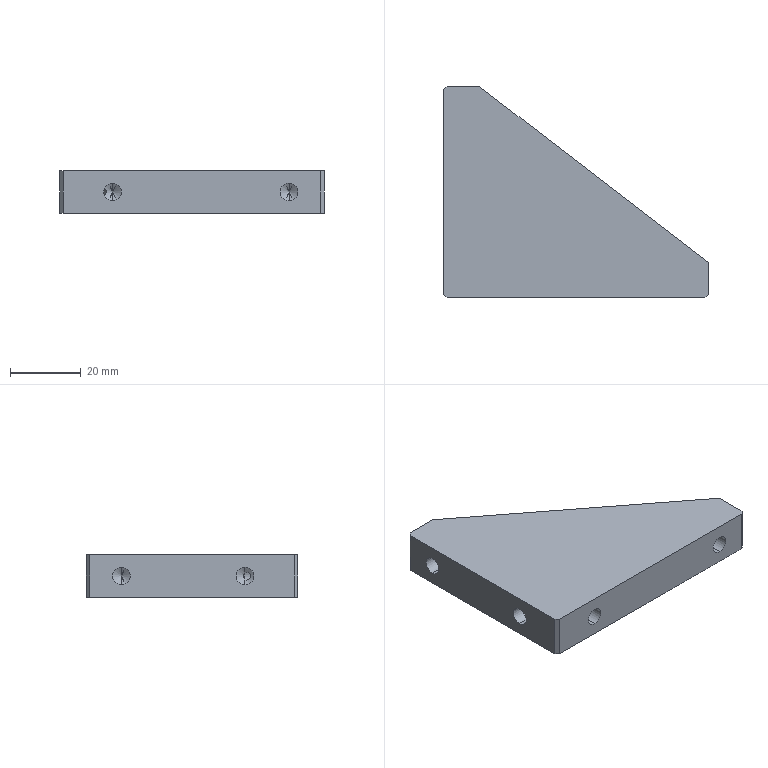Part | SolidWorks | features HoleWzd 2, Chamfer 1, Extrusion 1, ICE 1 | 1 solid | 26 faces | box 75 x 60 x 12 mm | volume 33384 mm3 | plane 10 | cone 8 | cylinder 8 | commonest cylinder face diameters 5 x8
STEP:
#1=CARTESIAN_POINT('',(-22.5,-13.498,0.));
#2=VERTEX_POINT('',#1);
#3=CARTESIAN_POINT('',(-22.5,-15.,-2.5));
#4=VERTEX_POINT('',#3);
#5=CARTESIAN_POINT('',(-22.5,-15.,-2.5));
#6=DIRECTION('',(0.,-0.515,-0.8572));
#7=VECTOR('',#6,1000.);
#8=LINE('',#5,#7);
#9=EDGE_CURVE('',#2,#4,#8,.T.);
#10=ORIENTED_EDGE('',*,*,#9,.F.);
#11=CARTESIAN_POINT('',(-22.5,-15.,2.5));
#12=VERTEX_POINT('',#11);
#13=CARTESIAN_POINT('',(-22.5,-15.,2.5));
#14=DIRECTION('',(0.,-0.515,0.8572));
#15=VECTOR('',#14,1000.);
#16=LINE('',#13,#15);
#17=EDGE_CURVE('',#2,#12,#16,.T.);
#18=ORIENTED_EDGE('',*,*,#17,.T.);
#19=CARTESIAN_POINT('',(-24.705,-15.,1.177));
#20=VERTEX_POINT('',#19);
#21=CARTESIAN_POINT('',(-22.5,-15.,0.));
#22=DIRECTION('',(0.,-1.,0.));
#23=DIRECTION('',(0.,0.,-1.));
#24=AXIS2_PLACEMENT_3D('',#21,#22,#23);
#25=CIRCLE('',#24,2.5);
#26=EDGE_CURVE('',#12,#20,#25,.T.);
#27=ORIENTED_EDGE('',*,*,#26,.T.);
#28=CARTESIAN_POINT('',(-24.705,-15.,-1.177));
#29=VERTEX_POINT('',#28);
#30=CARTESIAN_POINT('',(-24.705,-15.,-1.177));
#31=CARTESIAN_POINT('',(-24.601,-14.896,-1.004));
#32=CARTESIAN_POINT('',(-24.501,-14.795,-0.8272));
#33=CARTESIAN_POINT('',(-24.374,-14.668,-0.5368));
#34=CARTESIAN_POINT('',(-24.336,-14.63,-0.4366));
#35=CARTESIAN_POINT('',(-24.28,-14.574,-0.2236));
#36=CARTESIAN_POINT('',(-24.263,-14.557,-0.1115));
#37=CARTESIAN_POINT('',(-24.264,-14.558,0.1167));
#38=CARTESIAN_POINT('',(-24.281,-14.575,0.2286));
#39=CARTESIAN_POINT('',(-24.338,-14.632,0.4423));
#40=CARTESIAN_POINT('',(-24.376,-14.67,0.5413));
#41=CARTESIAN_POINT('',(-24.502,-14.796,0.8277));
#42=CARTESIAN_POINT('',(-24.602,-14.896,1.005));
#43=CARTESIAN_POINT('',(-24.705,-15.,1.177));
#44=B_SPLINE_CURVE_WITH_KNOTS('',3,(#30,#31,#32,#33,#34,#35,#36,#37,#38,#39,#40,#41,#42,#43),.UNSPECIFIED.,.F.,.F.,(4,2,2,2,2,2,4),(0.000000436,0.0006809,0.001021,0.001361,0.001702,0.002042,0.002722),.UNSPECIFIED.);
#45=EDGE_CURVE('',#29,#20,#44,.T.);
#46=ORIENTED_EDGE('',*,*,#45,.F.);
#47=CARTESIAN_POINT('',(-22.5,-15.,0.));
#48=DIRECTION('',(0.,-1.,0.));
#49=DIRECTION('',(0.,0.,-1.));
#50=AXIS2_PLACEMENT_3D('',#47,#48,#49);
#51=CIRCLE('',#50,2.5);
#52=EDGE_CURVE('',#29,#4,#51,.T.);
#53=ORIENTED_EDGE('',*,*,#52,.T.);
#54=EDGE_LOOP('',(#10,#18,#27,#46,#53));
#55=FACE_OUTER_BOUND('',#54,.T.);
#56=CARTESIAN_POINT('',(-22.5,-15.,0.));
#57=DIRECTION('',(0.,-1.,0.));
#58=DIRECTION('',(0.,0.,-1.));
#59=AXIS2_PLACEMENT_3D('',#56,#57,#58);
#60=CONICAL_SURFACE('',#59,2.5,1.03);
#61=ADVANCED_FACE('',(#55),#60,.F.);
#62=ORIENTED_EDGE('',*,*,#26,.F.);
#63=CARTESIAN_POINT('',(-22.5,-30.,2.5));
#64=VERTEX_POINT('',#63);
#65=CARTESIAN_POINT('',(-22.5,-30.,2.5));
#66=DIRECTION('',(0.,-1.,0.));
#67=VECTOR('',#66,1000.);
#68=LINE('',#65,#67);
#69=EDGE_CURVE('',#12,#64,#68,.T.);
#70=ORIENTED_EDGE('',*,*,#69,.T.);
#71=CARTESIAN_POINT('',(-22.5,-30.,-2.5));
#72=VERTEX_POINT('',#71);
#73=CARTESIAN_POINT('',(-22.5,-30.,0.));
#74=DIRECTION('',(0.,-1.,0.));
#75=DIRECTION('',(0.,0.,-1.));
#76=AXIS2_PLACEMENT_3D('',#73,#74,#75);
#77=CIRCLE('',#76,2.5);
#78=EDGE_CURVE('',#64,#72,#77,.T.);
#79=ORIENTED_EDGE('',*,*,#78,.T.);
#80=CARTESIAN_POINT('',(-22.5,-30.,-2.5));
#81=DIRECTION('',(0.,-1.,0.));
#82=VECTOR('',#81,1000.);
#83=LINE('',#80,#82);
#84=EDGE_CURVE('',#4,#72,#83,.T.);
#85=ORIENTED_EDGE('',*,*,#84,.F.);
#86=ORIENTED_EDGE('',*,*,#52,.F.);
#87=CARTESIAN_POINT('',(-24.705,-15.,1.177));
#88=CARTESIAN_POINT('',(-24.705,-15.188,1.177));
#89=CARTESIAN_POINT('',(-24.719,-15.377,1.153));
#90=CARTESIAN_POINT('',(-24.765,-15.738,1.058));
#91=CARTESIAN_POINT('',(-24.799,-15.911,0.9883));
#92=CARTESIAN_POINT('',(-24.854,-16.15,0.8446));
#93=CARTESIAN_POINT('',(-24.872,-16.225,0.7909));
#94=CARTESIAN_POINT('',(-24.91,-16.364,0.6694));
#95=CARTESIAN_POINT('',(-24.928,-16.429,0.6008));
#96=CARTESIAN_POINT('',(-24.96,-16.539,0.4508));
#97=CARTESIAN_POINT('',(-24.974,-16.586,0.3675));
#98=CARTESIAN_POINT('',(-24.994,-16.65,0.1905));
#99=CARTESIAN_POINT('',(-25.,-16.668,0.09531));
#100=CARTESIAN_POINT('',(-25.,-16.668,-0.09351));
#101=CARTESIAN_POINT('',(-24.994,-16.65,-0.1886));
#102=CARTESIAN_POINT('',(-24.975,-16.587,-0.3659));
#103=CARTESIAN_POINT('',(-24.96,-16.54,-0.4495));
#104=CARTESIAN_POINT('',(-24.912,-16.376,-0.6746));
#105=CARTESIAN_POINT('',(-24.872,-16.23,-0.7961));
#106=CARTESIAN_POINT('',(-24.799,-15.914,-0.9866));
#107=CARTESIAN_POINT('',(-24.766,-15.739,-1.058));
#108=CARTESIAN_POINT('',(-24.719,-15.378,-1.153));
#109=CARTESIAN_POINT('',(-24.705,-15.188,-1.177));
#110=CARTESIAN_POINT('',(-24.705,-15.,-1.177));
#111=B_SPLINE_CURVE_WITH_KNOTS('',3,(#87,#88,#89,#90,#91,#92,#93,#94,#95,#96,#97,#98,#99,#100,#101,#102,#103,#104,#105,#106,#107,#108,#109,#110),.UNSPECIFIED.,.F.,.F.,(4,2,2,2,2,2,2,2,2,2,2,4),(0.0002494,0.000812,0.001375,0.001656,0.001937,0.002219,0.0025,0.002781,0.003063,0.003625,0.004188,0.00475),.UNSPECIFIED.);
#112=EDGE_CURVE('',#20,#29,#111,.T.);
#113=ORIENTED_EDGE('',*,*,#112,.F.);
#114=EDGE_LOOP('',(#62,#70,#79,#85,#86,#113));
#115=FACE_OUTER_BOUND('',#114,.T.);
#116=CARTESIAN_POINT('',(-22.5,-30.,0.));
#117=DIRECTION('',(0.,-1.,0.));
#118=DIRECTION('',(0.,0.,-1.));
#119=AXIS2_PLACEMENT_3D('',#116,#117,#118);
#120=CYLINDRICAL_SURFACE('',#119,2.5);
#121=ADVANCED_FACE('',(#115),#120,.F.);
#122=CARTESIAN_POINT('',(27.5,-15.,2.5));
#123=VERTEX_POINT('',#122);
#124=CARTESIAN_POINT('',(27.5,-15.,-2.5));
#125=VERTEX_POINT('',#124);
#126=CARTESIAN_POINT('',(27.5,-15.,0.));
#127=DIRECTION('',(0.,-1.,0.));
#128=DIRECTION('',(0.,0.,-1.));
#129=AXIS2_PLACEMENT_3D('',#126,#127,#128);
#130=CIRCLE('',#129,2.5);
#131=EDGE_CURVE('',#123,#125,#130,.T.);
#132=ORIENTED_EDGE('',*,*,#131,.F.);
#133=CARTESIAN_POINT('',(27.5,-30.,2.5));
#134=VERTEX_POINT('',#133);
#135=CARTESIAN_POINT('',(27.5,-30.,2.5));
#136=DIRECTION('',(0.,-1.,0.));
#137=VECTOR('',#136,1000.);
#138=LINE('',#135,#137);
#139=EDGE_CURVE('',#123,#134,#138,.T.);
#140=ORIENTED_EDGE('',*,*,#139,.T.);
#141=CARTESIAN_POINT('',(27.5,-30.,-2.5));
#142=VERTEX_POINT('',#141);
#143=CARTESIAN_POINT('',(27.5,-30.,0.));
#144=DIRECTION('',(0.,-1.,0.));
#145=DIRECTION('',(0.,0.,-1.));
#146=AXIS2_PLACEMENT_3D('',#143,#144,#145);
#147=CIRCLE('',#146,2.5);
#148=EDGE_CURVE('',#134,#142,#147,.T.);
#149=ORIENTED_EDGE('',*,*,#148,.T.);
#150=CARTESIAN_POINT('',(27.5,-30.,-2.5));
#151=DIRECTION('',(0.,-1.,0.));
#152=VECTOR('',#151,1000.);
#153=LINE('',#150,#152);
#154=EDGE_CURVE('',#125,#142,#153,.T.);
#155=ORIENTED_EDGE('',*,*,#154,.F.);
#156=EDGE_LOOP('',(#132,#140,#149,#155));
#157=FACE_OUTER_BOUND('',#156,.T.);
#158=CARTESIAN_POINT('',(27.5,-30.,0.));
#159=DIRECTION('',(0.,-1.,0.));
#160=DIRECTION('',(0.,0.,-1.));
#161=AXIS2_PLACEMENT_3D('',#158,#159,#160);
#162=CYLINDRICAL_SURFACE('',#161,2.5);
#163=ADVANCED_FACE('',(#157),#162,.F.);
#164=CARTESIAN_POINT('',(27.5,-13.498,0.));
#165=VERTEX_POINT('',#164);
#166=CARTESIAN_POINT('',(27.5,-15.,-2.5));
#167=DIRECTION('',(0.,-0.515,-0.8572));
#168=VECTOR('',#167,1000.);
#169=LINE('',#166,#168);
#170=EDGE_CURVE('',#165,#125,#169,.T.);
#171=ORIENTED_EDGE('',*,*,#170,.F.);
#172=CARTESIAN_POINT('',(27.5,-15.,2.5));
#173=DIRECTION('',(0.,-0.515,0.8572));
#174=VECTOR('',#173,1000.);
#175=LINE('',#172,#174);
#176=EDGE_CURVE('',#165,#123,#175,.T.);
#177=ORIENTED_EDGE('',*,*,#176,.T.);
#178=ORIENTED_EDGE('',*,*,#131,.T.);
#179=EDGE_LOOP('',(#171,#177,#178));
#180=FACE_OUTER_BOUND('',#179,.T.);
#181=CARTESIAN_POINT('',(27.5,-15.,0.));
#182=DIRECTION('',(0.,-1.,0.));
#183=DIRECTION('',(0.,0.,-1.));
#184=AXIS2_PLACEMENT_3D('',#181,#182,#183);
#185=CONICAL_SURFACE('',#184,2.5,1.03);
#186=ADVANCED_FACE('',(#180),#185,.F.);
#187=CARTESIAN_POINT('',(-25.5,20.,-2.5));
#188=VERTEX_POINT('',#187);
#189=CARTESIAN_POINT('',(-25.5,20.,2.5));
#190=VERTEX_POINT('',#189);
#191=CARTESIAN_POINT('',(-25.5,20.,0.));
#192=DIRECTION('',(-1.,0.,0.));
#193=DIRECTION('',(0.,0.,1.));
#194=AXIS2_PLACEMENT_3D('',#191,#192,#193);
#195=CIRCLE('',#194,2.5);
#196=EDGE_CURVE('',#188,#190,#195,.T.);
#197=ORIENTED_EDGE('',*,*,#196,.F.);
#198=CARTESIAN_POINT('',(-37.5,20.,-2.5));
#199=VERTEX_POINT('',#198);
#200=CARTESIAN_POINT('',(-37.5,20.,-2.5));
#201=DIRECTION('',(-1.,0.,0.));
#202=VECTOR('',#201,1000.);
#203=LINE('',#200,#202);
#204=EDGE_CURVE('',#188,#199,#203,.T.);
#205=ORIENTED_EDGE('',*,*,#204,.T.);
#206=CARTESIAN_POINT('',(-37.5,20.,2.5));
#207=VERTEX_POINT('',#206);
#208=CARTESIAN_POINT('',(-37.5,20.,0.));
#209=DIRECTION('',(-1.,0.,0.));
#210=DIRECTION('',(0.,0.,1.));
#211=AXIS2_PLACEMENT_3D('',#208,#209,#210);
#212=CIRCLE('',#211,2.5);
#213=EDGE_CURVE('',#199,#207,#212,.T.);
#214=ORIENTED_EDGE('',*,*,#213,.T.);
#215=CARTESIAN_POINT('',(-37.5,20.,2.5));
#216=DIRECTION('',(-1.,0.,0.));
#217=VECTOR('',#216,1000.);
#218=LINE('',#215,#217);
#219=EDGE_CURVE('',#190,#207,#218,.T.);
#220=ORIENTED_EDGE('',*,*,#219,.F.);
#221=EDGE_LOOP('',(#197,#205,#214,#220));
#222=FACE_OUTER_BOUND('',#221,.T.);
#223=CARTESIAN_POINT('',(-37.5,20.,0.));
#224=DIRECTION('',(-1.,0.,0.));
#225=DIRECTION('',(0.,0.,1.));
#226=AXIS2_PLACEMENT_3D('',#223,#224,#225);
#227=CYLINDRICAL_SURFACE('',#226,2.5);
#228=ADVANCED_FACE('',(#222),#227,.F.);
#229=CARTESIAN_POINT('',(-23.998,20.,0.));
#230=VERTEX_POINT('',#229);
#231=CARTESIAN_POINT('',(-25.5,20.,2.5));
#232=DIRECTION('',(-0.515,0.,0.8572));
#233=VECTOR('',#232,1000.);
#234=LINE('',#231,#233);
#235=EDGE_CURVE('',#230,#190,#234,.T.);
#236=ORIENTED_EDGE('',*,*,#235,.F.);
#237=CARTESIAN_POINT('',(-25.5,20.,-2.5));
#238=DIRECTION('',(-0.515,0.,-0.8572));
#239=VECTOR('',#238,1000.);
#240=LINE('',#237,#239);
#241=EDGE_CURVE('',#230,#188,#240,.T.);
#242=ORIENTED_EDGE('',*,*,#241,.T.);
#243=ORIENTED_EDGE('',*,*,#196,.T.);
#244=EDGE_LOOP('',(#236,#242,#243));
#245=FACE_OUTER_BOUND('',#244,.T.);
#246=CARTESIAN_POINT('',(-25.5,20.,0.));
#247=DIRECTION('',(-1.,0.,0.));
#248=DIRECTION('',(0.,0.,1.));
#249=AXIS2_PLACEMENT_3D('',#246,#247,#248);
#250=CONICAL_SURFACE('',#249,2.5,1.03);
#251=ADVANCED_FACE('',(#245),#250,.F.);
#252=CARTESIAN_POINT('',(-25.5,-15.,-2.5));
#253=VERTEX_POINT('',#252);
#254=CARTESIAN_POINT('',(-25.5,-15.,2.5));
#255=VERTEX_POINT('',#254);
#256=CARTESIAN_POINT('',(-25.5,-15.,0.));
#257=DIRECTION('',(-1.,0.,0.));
#258=DIRECTION('',(0.,0.,1.));
#259=AXIS2_PLACEMENT_3D('',#256,#257,#258);
#260=CIRCLE('',#259,2.5);
#261=EDGE_CURVE('',#253,#255,#260,.T.);
#262=ORIENTED_EDGE('',*,*,#261,.F.);
#263=CARTESIAN_POINT('',(-37.5,-15.,-2.5));
#264=VERTEX_POINT('',#263);
#265=CARTESIAN_POINT('',(-37.5,-15.,-2.5));
#266=DIRECTION('',(-1.,0.,0.));
#267=VECTOR('',#266,1000.);
#268=LINE('',#265,#267);
#269=EDGE_CURVE('',#253,#264,#268,.T.);
#270=ORIENTED_EDGE('',*,*,#269,.T.);
#271=CARTESIAN_POINT('',(-37.5,-15.,2.5));
#272=VERTEX_POINT('',#271);
#273=CARTESIAN_POINT('',(-37.5,-15.,0.));
#274=DIRECTION('',(-1.,0.,0.));
#275=DIRECTION('',(0.,0.,1.));
#276=AXIS2_PLACEMENT_3D('',#273,#274,#275);
#277=CIRCLE('',#276,2.5);
#278=EDGE_CURVE('',#264,#272,#277,.T.);
#279=ORIENTED_EDGE('',*,*,#278,.T.);
#280=CARTESIAN_POINT('',(-37.5,-15.,2.5));
#281=DIRECTION('',(-1.,0.,0.));
#282=VECTOR('',#281,1000.);
#283=LINE('',#280,#282);
#284=EDGE_CURVE('',#255,#272,#283,.T.);
#285=ORIENTED_EDGE('',*,*,#284,.F.);
#286=EDGE_LOOP('',(#262,#270,#279,#285));
#287=FACE_OUTER_BOUND('',#286,.T.);
#288=CARTESIAN_POINT('',(-37.5,-15.,0.));
#289=DIRECTION('',(-1.,0.,0.));
#290=DIRECTION('',(0.,0.,1.));
#291=AXIS2_PLACEMENT_3D('',#288,#289,#290);
#292=CYLINDRICAL_SURFACE('',#291,2.5);
#293=ADVANCED_FACE('',(#287),#292,.F.);
#294=ORIENTED_EDGE('',*,*,#112,.T.);
#295=CARTESIAN_POINT('',(-25.5,-15.,-2.5));
#296=DIRECTION('',(-0.515,0.,-0.8572));
#297=VECTOR('',#296,1000.);
#298=LINE('',#295,#297);
#299=EDGE_CURVE('',#29,#253,#298,.T.);
#300=ORIENTED_EDGE('',*,*,#299,.T.);
#301=ORIENTED_EDGE('',*,*,#261,.T.);
#302=CARTESIAN_POINT('',(-25.5,-15.,2.5));
#303=DIRECTION('',(-0.515,0.,0.8572));
#304=VECTOR('',#303,1000.);
#305=LINE('',#302,#304);
#306=EDGE_CURVE('',#20,#255,#305,.T.);
#307=ORIENTED_EDGE('',*,*,#306,.F.);
#308=EDGE_LOOP('',(#294,#300,#301,#307));
#309=FACE_OUTER_BOUND('',#308,.T.);
#310=CARTESIAN_POINT('',(-25.5,-15.,0.));
#311=DIRECTION('',(-1.,0.,0.));
#312=DIRECTION('',(0.,0.,1.));
#313=AXIS2_PLACEMENT_3D('',#310,#311,#312);
#314=CONICAL_SURFACE('',#313,2.5,1.03);
#315=ADVANCED_FACE('',(#309),#314,.F.);
#316=CARTESIAN_POINT('',(37.5,-29.,6.));
#317=VERTEX_POINT('',#316);
#318=CARTESIAN_POINT('',(37.5,-20.,6.));
#319=VERTEX_POINT('',#318);
#320=CARTESIAN_POINT('',(37.5,30.,6.));
#321=DIRECTION('',(0.,1.,0.));
#322=VECTOR('',#321,1000.);
#323=LINE('',#320,#322);
#324=EDGE_CURVE('',#317,#319,#323,.T.);
#325=ORIENTED_EDGE('',*,*,#324,.F.);
#326=CARTESIAN_POINT('',(37.5,-29.,-6.));
#327=VERTEX_POINT('',#326);
#328=CARTESIAN_POINT('',(37.5,-29.,6.));
#329=DIRECTION('',(0.,0.,-1.));
#330=VECTOR('',#329,1000.);
#331=LINE('',#328,#330);
#332=EDGE_CURVE('',#317,#327,#331,.T.);
#333=ORIENTED_EDGE('',*,*,#332,.T.);
#334=CARTESIAN_POINT('',(37.5,-20.,-6.));
#335=VERTEX_POINT('',#334);
#336=CARTESIAN_POINT('',(37.5,30.,-6.));
#337=DIRECTION('',(0.,1.,0.));
#338=VECTOR('',#337,1000.);
#339=LINE('',#336,#338);
#340=EDGE_CURVE('',#327,#335,#339,.T.);
#341=ORIENTED_EDGE('',*,*,#340,.T.);
#342=CARTESIAN_POINT('',(37.5,-20.,-6.));
#343=DIRECTION('',(0.,0.,1.));
#344=VECTOR('',#343,1000.);
#345=LINE('',#342,#344);
#346=EDGE_CURVE('',#335,#319,#345,.T.);
#347=ORIENTED_EDGE('',*,*,#346,.T.);
#348=EDGE_LOOP('',(#325,#333,#341,#347));
#349=FACE_OUTER_BOUND('',#348,.T.);
#350=CARTESIAN_POINT('',(37.5,30.,6.));
#351=DIRECTION('',(-1.,0.,0.));
#352=DIRECTION('',(0.,-1.,0.));
#353=AXIS2_PLACEMENT_3D('',#350,#351,#352);
#354=PLANE('',#353);
#355=ADVANCED_FACE('',(#349),#354,.F.);
#356=CARTESIAN_POINT('',(-27.5,30.,-6.));
#357=VERTEX_POINT('',#356);
#358=CARTESIAN_POINT('',(-36.5,30.,-6.));
#359=VERTEX_POINT('',#358);
#360=CARTESIAN_POINT('',(-37.5,30.,-6.));
#361=DIRECTION('',(-1.,0.,0.));
#362=VECTOR('',#361,1000.);
#363=LINE('',#360,#362);
#364=EDGE_CURVE('',#357,#359,#363,.T.);
#365=ORIENTED_EDGE('',*,*,#364,.T.);
#366=CARTESIAN_POINT('',(-36.5,30.,6.));
#367=VERTEX_POINT('',#366);
#368=CARTESIAN_POINT('',(-36.5,30.,6.));
#369=DIRECTION('',(0.,0.,1.));
#370=VECTOR('',#369,1000.);
#371=LINE('',#368,#370);
#372=EDGE_CURVE('',#359,#367,#371,.T.);
#373=ORIENTED_EDGE('',*,*,#372,.T.);
#374=CARTESIAN_POINT('',(-27.5,30.,6.));
#375=VERTEX_POINT('',#374);
#376=CARTESIAN_POINT('',(-37.5,30.,6.));
#377=DIRECTION('',(-1.,0.,0.));
#378=VECTOR('',#377,1000.);
#379=LINE('',#376,#378);
#380=EDGE_CURVE('',#375,#367,#379,.T.);
#381=ORIENTED_EDGE('',*,*,#380,.F.);
#382=CARTESIAN_POINT('',(-27.5,30.,-6.));
#383=DIRECTION('',(0.,0.,1.));
#384=VECTOR('',#383,1000.);
#385=LINE('',#382,#384);
#386=EDGE_CURVE('',#357,#375,#385,.T.);
#387=ORIENTED_EDGE('',*,*,#386,.F.);
#388=EDGE_LOOP('',(#365,#373,#381,#387));
#389=FACE_OUTER_BOUND('',#388,.T.);
#390=CARTESIAN_POINT('',(-37.5,30.,6.));
#391=DIRECTION('',(0.,-1.,0.));
#392=DIRECTION('',(0.,0.,-1.));
#393=AXIS2_PLACEMENT_3D('',#390,#391,#392);
#394=PLANE('',#393);
#395=ADVANCED_FACE('',(#389),#394,.F.);
#396=CARTESIAN_POINT('',(-37.5,20.,0.));
#397=DIRECTION('',(-1.,0.,0.));
#398=DIRECTION('',(0.,0.,1.));
#399=AXIS2_PLACEMENT_3D('',#396,#397,#398);
#400=CIRCLE('',#399,2.5);
#401=EDGE_CURVE('',#207,#199,#400,.T.);
#402=ORIENTED_EDGE('',*,*,#401,.F.);
#403=ORIENTED_EDGE('',*,*,#213,.F.);
#404=EDGE_LOOP('',(#402,#403));
#405=FACE_BOUND('',#404,.T.);
#406=CARTESIAN_POINT('',(-37.5,-15.,0.));
#407=DIRECTION('',(-1.,0.,0.));
#408=DIRECTION('',(0.,0.,1.));
#409=AXIS2_PLACEMENT_3D('',#406,#407,#408);
#410=CIRCLE('',#409,2.5);
#411=EDGE_CURVE('',#272,#264,#410,.T.);
#412=ORIENTED_EDGE('',*,*,#411,.F.);
#413=ORIENTED_EDGE('',*,*,#278,.F.);
#414=EDGE_LOOP('',(#412,#413));
#415=FACE_BOUND('',#414,.T.);
#416=CARTESIAN_POINT('',(-37.5,29.,6.));
#417=VERTEX_POINT('',#416);
#418=CARTESIAN_POINT('',(-37.5,-29.,6.));
#419=VERTEX_POINT('',#418);
#420=CARTESIAN_POINT('',(-37.5,30.,6.));
#421=DIRECTION('',(0.,-1.,0.));
#422=VECTOR('',#421,1000.);
#423=LINE('',#420,#422);
#424=EDGE_CURVE('',#417,#419,#423,.T.);
#425=ORIENTED_EDGE('',*,*,#424,.F.);
#426=CARTESIAN_POINT('',(-37.5,29.,-6.));
#427=VERTEX_POINT('',#426);
#428=CARTESIAN_POINT('',(-37.5,29.,6.));
#429=DIRECTION('',(0.,0.,-1.));
#430=VECTOR('',#429,1000.);
#431=LINE('',#428,#430);
#432=EDGE_CURVE('',#417,#427,#431,.T.);
#433=ORIENTED_EDGE('',*,*,#432,.T.);
#434=CARTESIAN_POINT('',(-37.5,-29.,-6.));
#435=VERTEX_POINT('',#434);
#436=CARTESIAN_POINT('',(-37.5,30.,-6.));
#437=DIRECTION('',(0.,-1.,0.));
#438=VECTOR('',#437,1000.);
#439=LINE('',#436,#438);
#440=EDGE_CURVE('',#427,#435,#439,.T.);
#441=ORIENTED_EDGE('',*,*,#440,.T.);
#442=CARTESIAN_POINT('',(-37.5,-29.,6.));
#443=DIRECTION('',(0.,0.,1.));
#444=VECTOR('',#443,1000.);
#445=LINE('',#442,#444);
#446=EDGE_CURVE('',#435,#419,#445,.T.);
#447=ORIENTED_EDGE('',*,*,#446,.T.);
#448=EDGE_LOOP('',(#425,#433,#441,#447));
#449=FACE_OUTER_BOUND('',#448,.T.);
#450=CARTESIAN_POINT('',(-37.5,30.,6.));
#451=DIRECTION('',(1.,0.,0.));
#452=DIRECTION('',(0.,1.,0.));
#453=AXIS2_PLACEMENT_3D('',#450,#451,#452);
#454=PLANE('',#453);
#455=ADVANCED_FACE('',(#405,#415,#449),#454,.F.);
#456=CARTESIAN_POINT('',(-22.5,-30.,0.));
#457=DIRECTION('',(0.,-1.,0.));
#458=DIRECTION('',(0.,0.,-1.));
#459=AXIS2_PLACEMENT_3D('',#456,#457,#458);
#460=CIRCLE('',#459,2.5);
#461=EDGE_CURVE('',#72,#64,#460,.T.);
#462=ORIENTED_EDGE('',*,*,#461,.F.);
#463=ORIENTED_EDGE('',*,*,#78,.F.);
#464=EDGE_LOOP('',(#462,#463));
#465=FACE_BOUND('',#464,.T.);
#466=CARTESIAN_POINT('',(27.5,-30.,0.));
#467=DIRECTION('',(0.,-1.,0.));
#468=DIRECTION('',(0.,0.,-1.));
#469=AXIS2_PLACEMENT_3D('',#466,#467,#468);
#470=CIRCLE('',#469,2.5);
#471=EDGE_CURVE('',#142,#134,#470,.T.);
#472=ORIENTED_EDGE('',*,*,#471,.F.);
#473=ORIENTED_EDGE('',*,*,#148,.F.);
#474=EDGE_LOOP('',(#472,#473));
#475=FACE_BOUND('',#474,.T.);
#476=CARTESIAN_POINT('',(-36.5,-30.,-6.));
#477=VERTEX_POINT('',#476);
#478=CARTESIAN_POINT('',(36.5,-30.,-6.));
#479=VERTEX_POINT('',#478);
#480=CARTESIAN_POINT('',(-37.5,-30.,-6.));
#481=DIRECTION('',(1.,0.,0.));
#482=VECTOR('',#481,1000.);
#483=LINE('',#480,#482);
#484=EDGE_CURVE('',#477,#479,#483,.T.);
#485=ORIENTED_EDGE('',*,*,#484,.T.);
#486=CARTESIAN_POINT('',(36.5,-30.,6.));
#487=VERTEX_POINT('',#486);
#488=CARTESIAN_POINT('',(36.5,-30.,6.));
#489=DIRECTION('',(0.,0.,1.));
#490=VECTOR('',#489,1000.);
#491=LINE('',#488,#490);
#492=EDGE_CURVE('',#479,#487,#491,.T.);
#493=ORIENTED_EDGE('',*,*,#492,.T.);
#494=CARTESIAN_POINT('',(-36.5,-30.,6.));
#495=VERTEX_POINT('',#494);
#496=CARTESIAN_POINT('',(-37.5,-30.,6.));
#497=DIRECTION('',(1.,0.,0.));
#498=VECTOR('',#497,1000.);
#499=LINE('',#496,#498);
#500=EDGE_CURVE('',#495,#487,#499,.T.);
#501=ORIENTED_EDGE('',*,*,#500,.F.);
#502=CARTESIAN_POINT('',(-36.5,-30.,6.));
#503=DIRECTION('',(0.,0.,-1.));
#504=VECTOR('',#503,1000.);
#505=LINE('',#502,#504);
#506=EDGE_CURVE('',#495,#477,#505,.T.);
#507=ORIENTED_EDGE('',*,*,#506,.T.);
#508=EDGE_LOOP('',(#485,#493,#501,#507));
#509=FACE_OUTER_BOUND('',#508,.T.);
#510=CARTESIAN_POINT('',(-37.5,-30.,6.));
#511=DIRECTION('',(0.,1.,0.));
#512=DIRECTION('',(0.,0.,1.));
#513=AXIS2_PLACEMENT_3D('',#510,#511,#512);
#514=PLANE('',#513);
#515=ADVANCED_FACE('',(#465,#475,#509),#514,.F.);
#516=ORIENTED_EDGE('',*,*,#380,.T.);
#517=CARTESIAN_POINT('',(-33.25,33.25,6.));
#518=DIRECTION('',(-0.7071,-0.7071,0.));
#519=VECTOR('',#518,1000.);
#520=LINE('',#517,#519);
#521=EDGE_CURVE('',#367,#417,#520,.T.);
#522=ORIENTED_EDGE('',*,*,#521,.T.);
#523=ORIENTED_EDGE('',*,*,#424,.T.);
#524=CARTESIAN_POINT('',(-33.25,-33.25,6.));
#525=DIRECTION('',(0.7071,-0.7071,0.));
#526=VECTOR('',#525,1000.);
#527=LINE('',#524,#526);
#528=EDGE_CURVE('',#419,#495,#527,.T.);
#529=ORIENTED_EDGE('',*,*,#528,.T.);
#530=ORIENTED_EDGE('',*,*,#500,.T.);
#531=CARTESIAN_POINT('',(33.25,-33.25,6.));
#532=DIRECTION('',(0.7071,0.7071,0.));
#533=VECTOR('',#532,1000.);
#534=LINE('',#531,#533);
#535=EDGE_CURVE('',#487,#317,#534,.T.);
#536=ORIENTED_EDGE('',*,*,#535,.T.);
#537=ORIENTED_EDGE('',*,*,#324,.T.);
#538=CARTESIAN_POINT('',(-27.5,30.,6.));
#539=DIRECTION('',(0.7926,-0.6097,0.));
#540=VECTOR('',#539,1000.);
#541=LINE('',#538,#540);
#542=EDGE_CURVE('',#375,#319,#541,.T.);
#543=ORIENTED_EDGE('',*,*,#542,.F.);
#544=EDGE_LOOP('',(#516,#522,#523,#529,#530,#536,#537,#543));
#545=FACE_OUTER_BOUND('',#544,.T.);
#546=CARTESIAN_POINT('',(0.,0.,6.));
#547=DIRECTION('',(0.,0.,1.));
#548=DIRECTION('',(1.,0.,0.));
#549=AXIS2_PLACEMENT_3D('',#546,#547,#548);
#550=PLANE('',#549);
#551=ADVANCED_FACE('',(#545),#550,.T.);
#552=ORIENTED_EDGE('',*,*,#440,.F.);
#553=CARTESIAN_POINT('',(-37.5,29.,-6.));
#554=DIRECTION('',(0.7071,0.7071,0.));
#555=VECTOR('',#554,1000.);
#556=LINE('',#553,#555);
#557=EDGE_CURVE('',#427,#359,#556,.T.);
#558=ORIENTED_EDGE('',*,*,#557,.T.);
#559=ORIENTED_EDGE('',*,*,#364,.F.);
#560=CARTESIAN_POINT('',(-27.5,30.,-6.));
#561=DIRECTION('',(0.7926,-0.6097,0.));
#562=VECTOR('',#561,1000.);
#563=LINE('',#560,#562);
#564=EDGE_CURVE('',#357,#335,#563,.T.);
#565=ORIENTED_EDGE('',*,*,#564,.T.);
#566=ORIENTED_EDGE('',*,*,#340,.F.);
#567=CARTESIAN_POINT('',(37.5,-29.,-6.));
#568=DIRECTION('',(-0.7071,-0.7071,0.));
#569=VECTOR('',#568,1000.);
#570=LINE('',#567,#569);
#571=EDGE_CURVE('',#327,#479,#570,.T.);
#572=ORIENTED_EDGE('',*,*,#571,.T.);
#573=ORIENTED_EDGE('',*,*,#484,.F.);
#574=CARTESIAN_POINT('',(-36.5,-30.,-6.));
#575=DIRECTION('',(-0.7071,0.7071,0.));
#576=VECTOR('',#575,1000.);
#577=LINE('',#574,#576);
#578=EDGE_CURVE('',#477,#435,#577,.T.);
#579=ORIENTED_EDGE('',*,*,#578,.T.);
#580=EDGE_LOOP('',(#552,#558,#559,#565,#566,#572,#573,#579));
#581=FACE_OUTER_BOUND('',#580,.T.);
#582=CARTESIAN_POINT('',(0.,0.,-6.));
#583=DIRECTION('',(0.,0.,1.));
#584=DIRECTION('',(1.,0.,0.));
#585=AXIS2_PLACEMENT_3D('',#582,#583,#584);
#586=PLANE('',#585);
#587=ADVANCED_FACE('',(#581),#586,.F.);
#588=ORIENTED_EDGE('',*,*,#542,.T.);
#589=ORIENTED_EDGE('',*,*,#346,.F.);
#590=ORIENTED_EDGE('',*,*,#564,.F.);
#591=ORIENTED_EDGE('',*,*,#386,.T.);
#592=EDGE_LOOP('',(#588,#589,#590,#591));
#593=FACE_OUTER_BOUND('',#592,.T.);
#594=CARTESIAN_POINT('',(-27.5,30.,-6.));
#595=DIRECTION('',(-0.6097,-0.7926,0.));
#596=DIRECTION('',(0.7926,-0.6097,0.));
#597=AXIS2_PLACEMENT_3D('',#594,#595,#596);
#598=PLANE('',#597);
#599=ADVANCED_FACE('',(#593),#598,.F.);
#600=ORIENTED_EDGE('',*,*,#299,.F.);
#601=ORIENTED_EDGE('',*,*,#45,.T.);
#602=ORIENTED_EDGE('',*,*,#306,.T.);
#603=CARTESIAN_POINT('',(-25.5,-15.,0.));
#604=DIRECTION('',(-1.,0.,0.));
#605=DIRECTION('',(0.,0.,1.));
#606=AXIS2_PLACEMENT_3D('',#603,#604,#605);
#607=CIRCLE('',#606,2.5);
#608=EDGE_CURVE('',#255,#253,#607,.T.);
#609=ORIENTED_EDGE('',*,*,#608,.T.);
#610=EDGE_LOOP('',(#600,#601,#602,#609));
#611=FACE_OUTER_BOUND('',#610,.T.);
#612=CARTESIAN_POINT('',(-25.5,-15.,0.));
#613=DIRECTION('',(-1.,0.,0.));
#614=DIRECTION('',(0.,0.,1.));
#615=AXIS2_PLACEMENT_3D('',#612,#613,#614);
#616=CONICAL_SURFACE('',#615,2.5,1.03);
#617=ADVANCED_FACE('',(#611),#616,.F.);
#618=ORIENTED_EDGE('',*,*,#269,.F.);
#619=ORIENTED_EDGE('',*,*,#608,.F.);
#620=ORIENTED_EDGE('',*,*,#284,.T.);
#621=ORIENTED_EDGE('',*,*,#411,.T.);
#622=EDGE_LOOP('',(#618,#619,#620,#621));
#623=FACE_OUTER_BOUND('',#622,.T.);
#624=CARTESIAN_POINT('',(-37.5,-15.,0.));
#625=DIRECTION('',(-1.,0.,0.));
#626=DIRECTION('',(0.,0.,1.));
#627=AXIS2_PLACEMENT_3D('',#624,#625,#626);
#628=CYLINDRICAL_SURFACE('',#627,2.5);
#629=ADVANCED_FACE('',(#623),#628,.F.);
#630=ORIENTED_EDGE('',*,*,#241,.F.);
#631=ORIENTED_EDGE('',*,*,#235,.T.);
#632=CARTESIAN_POINT('',(-25.5,20.,0.));
#633=DIRECTION('',(-1.,0.,0.));
#634=DIRECTION('',(0.,0.,1.));
#635=AXIS2_PLACEMENT_3D('',#632,#633,#634);
#636=CIRCLE('',#635,2.5);
#637=EDGE_CURVE('',#190,#188,#636,.T.);
#638=ORIENTED_EDGE('',*,*,#637,.T.);
#639=EDGE_LOOP('',(#630,#631,#638));
#640=FACE_OUTER_BOUND('',#639,.T.);
#641=CARTESIAN_POINT('',(-25.5,20.,0.));
#642=DIRECTION('',(-1.,0.,0.));
#643=DIRECTION('',(0.,0.,1.));
#644=AXIS2_PLACEMENT_3D('',#641,#642,#643);
#645=CONICAL_SURFACE('',#644,2.5,1.03);
#646=ADVANCED_FACE('',(#640),#645,.F.);
#647=ORIENTED_EDGE('',*,*,#204,.F.);
#648=ORIENTED_EDGE('',*,*,#637,.F.);
#649=ORIENTED_EDGE('',*,*,#219,.T.);
#650=ORIENTED_EDGE('',*,*,#401,.T.);
#651=EDGE_LOOP('',(#647,#648,#649,#650));
#652=FACE_OUTER_BOUND('',#651,.T.);
#653=CARTESIAN_POINT('',(-37.5,20.,0.));
#654=DIRECTION('',(-1.,0.,0.));
#655=DIRECTION('',(0.,0.,1.));
#656=AXIS2_PLACEMENT_3D('',#653,#654,#655);
#657=CYLINDRICAL_SURFACE('',#656,2.5);
#658=ADVANCED_FACE('',(#652),#657,.F.);
#659=ORIENTED_EDGE('',*,*,#176,.F.);
#660=ORIENTED_EDGE('',*,*,#170,.T.);
#661=CARTESIAN_POINT('',(27.5,-15.,0.));
#662=DIRECTION('',(0.,-1.,0.));
#663=DIRECTION('',(0.,0.,-1.));
#664=AXIS2_PLACEMENT_3D('',#661,#662,#663);
#665=CIRCLE('',#664,2.5);
#666=EDGE_CURVE('',#125,#123,#665,.T.);
#667=ORIENTED_EDGE('',*,*,#666,.T.);
#668=EDGE_LOOP('',(#659,#660,#667));
#669=FACE_OUTER_BOUND('',#668,.T.);
#670=CARTESIAN_POINT('',(27.5,-15.,0.));
#671=DIRECTION('',(0.,-1.,0.));
#672=DIRECTION('',(0.,0.,-1.));
#673=AXIS2_PLACEMENT_3D('',#670,#671,#672);
#674=CONICAL_SURFACE('',#673,2.5,1.03);
#675=ADVANCED_FACE('',(#669),#674,.F.);
#676=ORIENTED_EDGE('',*,*,#139,.F.);
#677=ORIENTED_EDGE('',*,*,#666,.F.);
#678=ORIENTED_EDGE('',*,*,#154,.T.);
#679=ORIENTED_EDGE('',*,*,#471,.T.);
#680=EDGE_LOOP('',(#676,#677,#678,#679));
#681=FACE_OUTER_BOUND('',#680,.T.);
#682=CARTESIAN_POINT('',(27.5,-30.,0.));
#683=DIRECTION('',(0.,-1.,0.));
#684=DIRECTION('',(0.,0.,-1.));
#685=AXIS2_PLACEMENT_3D('',#682,#683,#684);
#686=CYLINDRICAL_SURFACE('',#685,2.5);
#687=ADVANCED_FACE('',(#681),#686,.F.);
#688=ORIENTED_EDGE('',*,*,#69,.F.);
#689=CARTESIAN_POINT('',(-22.5,-15.,0.));
#690=DIRECTION('',(0.,-1.,0.));
#691=DIRECTION('',(0.,0.,-1.));
#692=AXIS2_PLACEMENT_3D('',#689,#690,#691);
#693=CIRCLE('',#692,2.5);
#694=EDGE_CURVE('',#4,#12,#693,.T.);
#695=ORIENTED_EDGE('',*,*,#694,.F.);
#696=ORIENTED_EDGE('',*,*,#84,.T.);
#697=ORIENTED_EDGE('',*,*,#461,.T.);
#698=EDGE_LOOP('',(#688,#695,#696,#697));
#699=FACE_OUTER_BOUND('',#698,.T.);
#700=CARTESIAN_POINT('',(-22.5,-30.,0.));
#701=DIRECTION('',(0.,-1.,0.));
#702=DIRECTION('',(0.,0.,-1.));
#703=AXIS2_PLACEMENT_3D('',#700,#701,#702);
#704=CYLINDRICAL_SURFACE('',#703,2.5);
#705=ADVANCED_FACE('',(#699),#704,.F.);
#706=ORIENTED_EDGE('',*,*,#17,.F.);
#707=ORIENTED_EDGE('',*,*,#9,.T.);
#708=ORIENTED_EDGE('',*,*,#694,.T.);
#709=EDGE_LOOP('',(#706,#707,#708));
#710=FACE_OUTER_BOUND('',#709,.T.);
#711=CARTESIAN_POINT('',(-22.5,-15.,0.));
#712=DIRECTION('',(0.,-1.,0.));
#713=DIRECTION('',(0.,0.,-1.));
#714=AXIS2_PLACEMENT_3D('',#711,#712,#713);
#715=CONICAL_SURFACE('',#714,2.5,1.03);
#716=ADVANCED_FACE('',(#710),#715,.F.);
#717=ORIENTED_EDGE('',*,*,#521,.F.);
#718=ORIENTED_EDGE('',*,*,#372,.F.);
#719=ORIENTED_EDGE('',*,*,#557,.F.);
#720=ORIENTED_EDGE('',*,*,#432,.F.);
#721=EDGE_LOOP('',(#717,#718,#719,#720));
#722=FACE_OUTER_BOUND('',#721,.T.);
#723=CARTESIAN_POINT('',(-37.5,29.,6.));
#724=DIRECTION('',(0.7071,-0.7071,0.));
#725=DIRECTION('',(0.,0.,-1.));
#726=AXIS2_PLACEMENT_3D('',#723,#724,#725);
#727=PLANE('',#726);
#728=ADVANCED_FACE('',(#722),#727,.F.);
#729=ORIENTED_EDGE('',*,*,#535,.F.);
#730=ORIENTED_EDGE('',*,*,#492,.F.);
#731=ORIENTED_EDGE('',*,*,#571,.F.);
#732=ORIENTED_EDGE('',*,*,#332,.F.);
#733=EDGE_LOOP('',(#729,#730,#731,#732));
#734=FACE_OUTER_BOUND('',#733,.T.);
#735=CARTESIAN_POINT('',(37.5,-29.,6.));
#736=DIRECTION('',(-0.7071,0.7071,0.));
#737=DIRECTION('',(0.,0.,-1.));
#738=AXIS2_PLACEMENT_3D('',#735,#736,#737);
#739=PLANE('',#738);
#740=ADVANCED_FACE('',(#734),#739,.F.);
#741=ORIENTED_EDGE('',*,*,#528,.F.);
#742=ORIENTED_EDGE('',*,*,#446,.F.);
#743=ORIENTED_EDGE('',*,*,#578,.F.);
#744=ORIENTED_EDGE('',*,*,#506,.F.);
#745=EDGE_LOOP('',(#741,#742,#743,#744));
#746=FACE_OUTER_BOUND('',#745,.T.);
#747=CARTESIAN_POINT('',(-36.5,-30.,6.));
#748=DIRECTION('',(0.7071,0.7071,0.));
#749=DIRECTION('',(0.,0.,-1.));
#750=AXIS2_PLACEMENT_3D('',#747,#748,#749);
#751=PLANE('',#750);
#752=ADVANCED_FACE('',(#746),#751,.F.);
#753=CLOSED_SHELL('',(#61,#121,#163,#186,#228,#251,#293,#315,#355,#395,#455,#515,#551,#587,#599,#617,#629,#646,#658,#675,#687,#705,#716,#728,#740,#752));
#754=MANIFOLD_SOLID_BREP('',#753);
#755=CARTESIAN_POINT('',(0.,0.,0.));
#756=DIRECTION('',(0.,0.,1.));
#757=DIRECTION('',(1.,0.,0.));
#758=AXIS2_PLACEMENT_3D('',#755,#756,#757);
#759=(LENGTH_UNIT()NAMED_UNIT(*)SI_UNIT(.MILLI.,.METRE.));
#760=UNCERTAINTY_MEASURE_WITH_UNIT(LENGTH_MEASURE(0.00001),#759,'','');
#761=(NAMED_UNIT(*)PLANE_ANGLE_UNIT()SI_UNIT($,.RADIAN.));
#762=(NAMED_UNIT(*)SI_UNIT($,.STERADIAN.)SOLID_ANGLE_UNIT());
#763=(GEOMETRIC_REPRESENTATION_CONTEXT(3)GLOBAL_UNCERTAINTY_ASSIGNED_CONTEXT((#760))GLOBAL_UNIT_ASSIGNED_CONTEXT((#759,#761,#762))REPRESENTATION_CONTEXT('',''));
#764=ADVANCED_BREP_SHAPE_REPRESENTATION('',(#754,#758),#763);